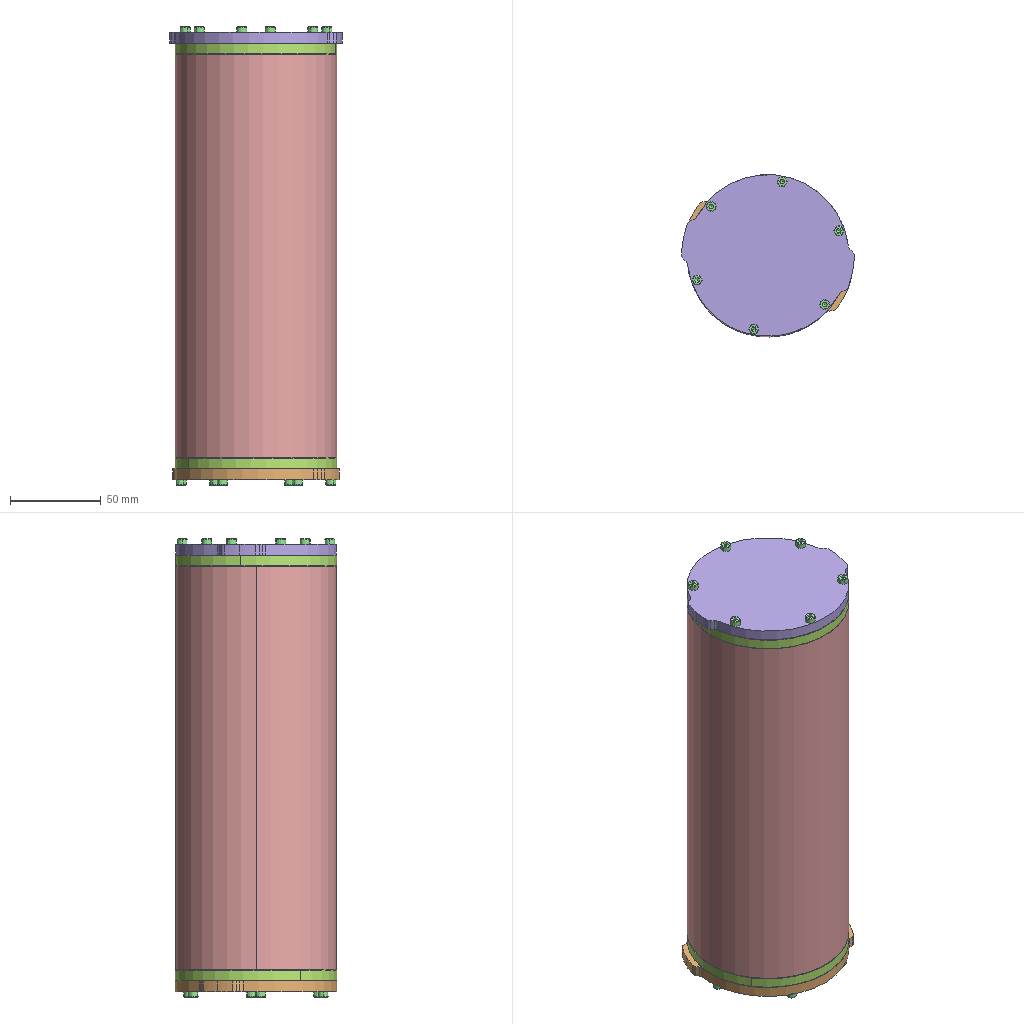Assembly | SolidWorks | 10 different items | 15 placed | box 95 x 89 x 252 mm
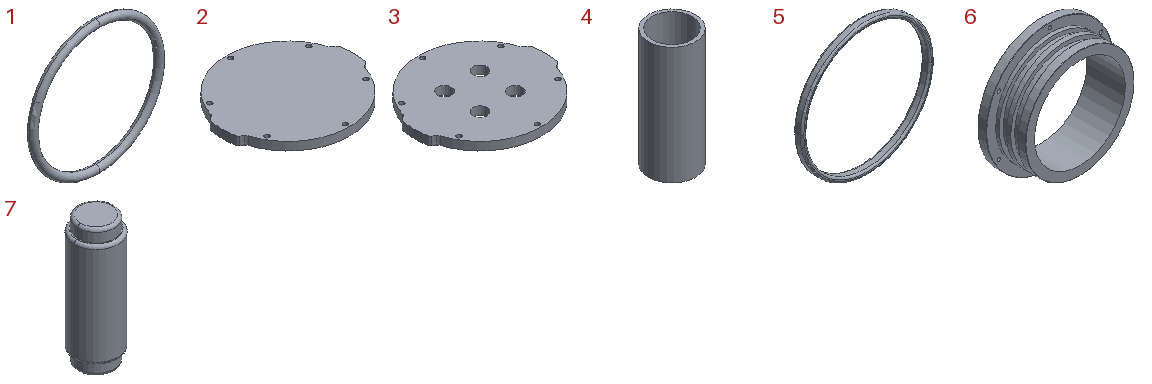Parts list (item | name | quantity | size | volume | features):
1 | - | x2 | 76.75 x 4.5 x 76.75 mm | 3610 mm3 | features Revolution 1
2 | - | x1 | 94.9 x 88.9 x 6 mm | 37769 mm3 | features Extrusion 1
3 | - | x1 | 94.9 x 88.9 x 6 mm | 35808 mm3 | features Extrusion 1
4 | - | x1 | 88.9 x 88.9 x 222 mm | 365589 mm3 | features Extrusion 1
5 | - | x4 | 75.946 x 4.826 x 75.946 mm | 2793 mm3 | features Revolution 1
6 | - | x2 | 88.9 x 27 x 88.9 mm | 39147 mm3 | features Chamfer 2, HoleWzd 1, ICE 1, Revolution 1
7 | - | x1 | 76 x 76 x 222 mm | 934259 mm3 | features ICE 3, Extrusion 1, Fillet 1
8 | hexagon socket head cap screws gb | x1 | - | - | -
9 | Waterproof terminal | x1 | - | - | -
10 | Waterproof terminal nut | x1 | - | - | -
Mates (type | each side: item.copy, entity, surface, feature):
Concentric | 4.1 face cylinder Boss-Extrude1 | 7.1 face cylinder Boss-Extrude1
Coincident | 4.1 face plane Boss-Extrude1 | 7.1 face plane Boss-Extrude1
Concentric | 4.1 face cylinder Boss-Extrude1 | 6.1 face cylinder Revolve1
Concentric | 6.1 face cylinder Revolve1 | 5.1 face cylinder Revolve1
Coincident | 6.1 face plane Revolve1 | 5.1 face plane Revolve1
Concentric | 6.1 face cylinder Revolve1 | 5.2 face cylinder Revolve1
Coincident | 6.1 face plane Revolve1 | 5.2 face plane Revolve1
Coincident | 4.1 face plane Boss-Extrude1 | 6.1 face plane Revolve1
Concentric | 6.2 face cylinder Revolve1 | 5.3 face cylinder Revolve1
Concentric | 6.2 face cylinder Revolve1 | 5.4 face cylinder Revolve1
Coincident | 6.2 face plane Revolve1 | 5.4 face plane Revolve1
Coincident | 6.2 face plane Revolve1 | 5.3 face plane Revolve1
Concentric | 4.1 face cylinder Boss-Extrude1 | 6.2 face cylinder Revolve1
Coincident | 4.1 face plane Boss-Extrude1 | 6.2 face plane Revolve1
Tangent | 6.1 face plane Cut-Extrude1 | 1.1 face torus Revolve1
Concentric | 4.1 face cylinder Boss-Extrude1 | 1.1 select_type:24
Concentric | 4.1 face cylinder Boss-Extrude1 | 1.2 select_type:24
Tangent | 6.2 face plane Cut-Extrude1 | 1.2 face torus Revolve1
Concentric | 4.1 face cylinder Boss-Extrude1 | 3.1 face cylinder Boss-Extrude1
Coincident | 6.2 face plane Revolve1 | 3.1 face plane Boss-Extrude1
Concentric | 6.2 face cylinder M3 Tapped Hole1 | 3.1 face cylinder Boss-Extrude1
Coincident | 6.1 face plane Revolve1 | 2.1 face plane Boss-Extrude1
Concentric | 4.1 face cylinder Boss-Extrude1 | 2.1 face cylinder Boss-Extrude1
Concentric | 6.1 face cylinder M3 Tapped Hole1 | 2.1 face cylinder Boss-Extrude1